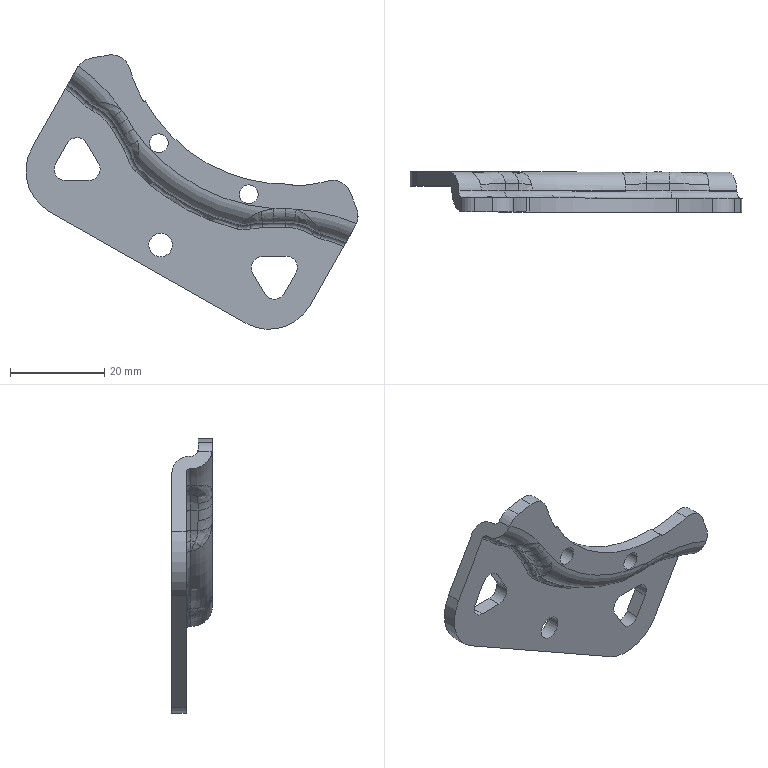Part | NX | features BREP 1 | 1 solid | 160 faces | box 70.641 x 8.571 x 58.399 mm | volume 6063 mm3 | cylinder 53 | torus 34 | plane 33 | spline 28 | cone 12 | commonest cylinder face diameters 0.6 x12 4.8 x6 4 x4 8 x4 10 x4 22 x4